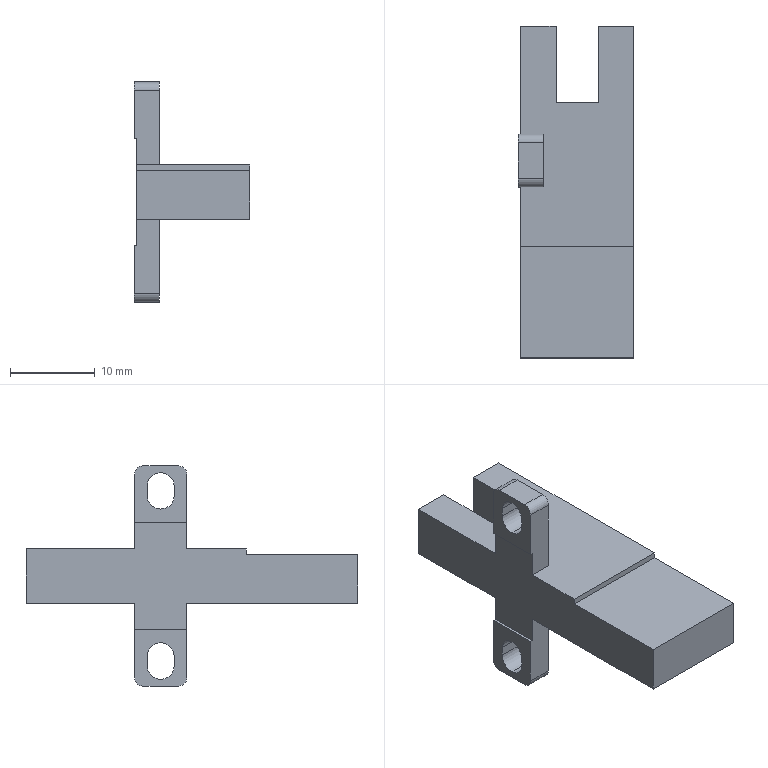Part | SolidWorks | features BaseBody 1 | 1 solid | 38 faces | box 13.7 x 39.2 x 26 mm | volume 3231 mm3 | plane 28 | cylinder 10 | commonest cylinder face diameters 3.2 x6 2 x4
STEP:
#1=CARTESIAN_POINT('',(-7.,6.3,-12.2));
#2=VERTEX_POINT('',#1);
#3=CARTESIAN_POINT('',(-7.,7.9,-10.6));
#4=VERTEX_POINT('',#3);
#5=CARTESIAN_POINT('',(-7.,6.3,-10.6));
#6=DIRECTION('',(1.,0.,0.));
#7=DIRECTION('',(0.,0.,-1.));
#8=AXIS2_PLACEMENT_3D('',#5,#6,#7);
#9=CIRCLE('',#8,1.6);
#10=EDGE_CURVE('',#2,#4,#9,.T.);
#11=ORIENTED_EDGE('',*,*,#10,.F.);
#12=CARTESIAN_POINT('',(-4.,6.3,-12.2));
#13=VERTEX_POINT('',#12);
#14=CARTESIAN_POINT('',(-4.,6.3,-12.2));
#15=DIRECTION('',(1.,0.,0.));
#16=VECTOR('',#15,1000.);
#17=LINE('',#14,#16);
#18=EDGE_CURVE('',#2,#13,#17,.T.);
#19=ORIENTED_EDGE('',*,*,#18,.T.);
#20=CARTESIAN_POINT('',(-4.,7.9,-10.6));
#21=VERTEX_POINT('',#20);
#22=CARTESIAN_POINT('',(-4.,6.3,-10.6));
#23=DIRECTION('',(-1.,0.,0.));
#24=DIRECTION('',(0.,0.,-1.));
#25=AXIS2_PLACEMENT_3D('',#22,#23,#24);
#26=CIRCLE('',#25,1.6);
#27=EDGE_CURVE('',#21,#13,#26,.T.);
#28=ORIENTED_EDGE('',*,*,#27,.F.);
#29=CARTESIAN_POINT('',(-4.,7.9,-10.6));
#30=DIRECTION('',(1.,0.,0.));
#31=VECTOR('',#30,1000.);
#32=LINE('',#29,#31);
#33=EDGE_CURVE('',#4,#21,#32,.T.);
#34=ORIENTED_EDGE('',*,*,#33,.F.);
#35=EDGE_LOOP('',(#11,#19,#28,#34));
#36=FACE_OUTER_BOUND('',#35,.T.);
#37=CARTESIAN_POINT('',(-4.,6.3,-10.6));
#38=DIRECTION('',(1.,0.,0.));
#39=DIRECTION('',(0.,0.,-1.));
#40=AXIS2_PLACEMENT_3D('',#37,#38,#39);
#41=CYLINDRICAL_SURFACE('',#40,1.6);
#42=ADVANCED_FACE('',(#36),#41,.F.);
#43=CARTESIAN_POINT('',(-7.,6.3,7.9));
#44=VERTEX_POINT('',#43);
#45=CARTESIAN_POINT('',(-7.,7.9,9.5));
#46=VERTEX_POINT('',#45);
#47=CARTESIAN_POINT('',(-7.,6.3,9.5));
#48=DIRECTION('',(1.,0.,0.));
#49=DIRECTION('',(0.,0.,-1.));
#50=AXIS2_PLACEMENT_3D('',#47,#48,#49);
#51=CIRCLE('',#50,1.6);
#52=EDGE_CURVE('',#44,#46,#51,.T.);
#53=ORIENTED_EDGE('',*,*,#52,.F.);
#54=CARTESIAN_POINT('',(-4.,6.3,7.9));
#55=VERTEX_POINT('',#54);
#56=CARTESIAN_POINT('',(-4.,6.3,7.9));
#57=DIRECTION('',(1.,0.,0.));
#58=VECTOR('',#57,1000.);
#59=LINE('',#56,#58);
#60=EDGE_CURVE('',#44,#55,#59,.T.);
#61=ORIENTED_EDGE('',*,*,#60,.T.);
#62=CARTESIAN_POINT('',(-4.,7.9,9.5));
#63=VERTEX_POINT('',#62);
#64=CARTESIAN_POINT('',(-4.,6.3,9.5));
#65=DIRECTION('',(-1.,0.,0.));
#66=DIRECTION('',(0.,0.,-1.));
#67=AXIS2_PLACEMENT_3D('',#64,#65,#66);
#68=CIRCLE('',#67,1.6);
#69=EDGE_CURVE('',#63,#55,#68,.T.);
#70=ORIENTED_EDGE('',*,*,#69,.F.);
#71=CARTESIAN_POINT('',(-4.,7.9,9.5));
#72=DIRECTION('',(1.,0.,0.));
#73=VECTOR('',#72,1000.);
#74=LINE('',#71,#73);
#75=EDGE_CURVE('',#46,#63,#74,.T.);
#76=ORIENTED_EDGE('',*,*,#75,.F.);
#77=EDGE_LOOP('',(#53,#61,#70,#76));
#78=FACE_OUTER_BOUND('',#77,.T.);
#79=CARTESIAN_POINT('',(-4.,6.3,9.5));
#80=DIRECTION('',(1.,0.,0.));
#81=DIRECTION('',(0.,0.,-1.));
#82=AXIS2_PLACEMENT_3D('',#79,#80,#81);
#83=CYLINDRICAL_SURFACE('',#82,1.6);
#84=ADVANCED_FACE('',(#78),#83,.F.);
#85=CARTESIAN_POINT('',(2.5,22.2,-3.2));
#86=VERTEX_POINT('',#85);
#87=CARTESIAN_POINT('',(2.5,13.2,-3.2));
#88=VERTEX_POINT('',#87);
#89=CARTESIAN_POINT('',(2.5,0.,-3.2));
#90=DIRECTION('',(0.,-1.,0.));
#91=VECTOR('',#90,1000.);
#92=LINE('',#89,#91);
#93=EDGE_CURVE('',#86,#88,#92,.T.);
#94=ORIENTED_EDGE('',*,*,#93,.F.);
#95=CARTESIAN_POINT('',(6.7,22.2,-3.2));
#96=VERTEX_POINT('',#95);
#97=CARTESIAN_POINT('',(0.,22.2,-3.2));
#98=DIRECTION('',(-1.,0.,0.));
#99=VECTOR('',#98,1000.);
#100=LINE('',#97,#99);
#101=EDGE_CURVE('',#96,#86,#100,.T.);
#102=ORIENTED_EDGE('',*,*,#101,.F.);
#103=CARTESIAN_POINT('',(6.7,-17.,-3.2));
#104=VERTEX_POINT('',#103);
#105=CARTESIAN_POINT('',(6.7,0.,-3.2));
#106=DIRECTION('',(0.,1.,0.));
#107=VECTOR('',#106,1000.);
#108=LINE('',#105,#107);
#109=EDGE_CURVE('',#104,#96,#108,.T.);
#110=ORIENTED_EDGE('',*,*,#109,.F.);
#111=CARTESIAN_POINT('',(-6.7,-17.,-3.2));
#112=VERTEX_POINT('',#111);
#113=CARTESIAN_POINT('',(0.,-17.,-3.2));
#114=DIRECTION('',(1.,0.,0.));
#115=VECTOR('',#114,1000.);
#116=LINE('',#113,#115);
#117=EDGE_CURVE('',#112,#104,#116,.T.);
#118=ORIENTED_EDGE('',*,*,#117,.F.);
#119=CARTESIAN_POINT('',(-6.7,3.2,-3.2));
#120=VERTEX_POINT('',#119);
#121=CARTESIAN_POINT('',(-6.7,0.,-3.2));
#122=DIRECTION('',(0.,-1.,0.));
#123=VECTOR('',#122,1000.);
#124=LINE('',#121,#123);
#125=EDGE_CURVE('',#120,#112,#124,.T.);
#126=ORIENTED_EDGE('',*,*,#125,.F.);
#127=CARTESIAN_POINT('',(-4.,3.2,-3.2));
#128=VERTEX_POINT('',#127);
#129=CARTESIAN_POINT('',(0.,3.2,-3.2));
#130=DIRECTION('',(-1.,0.,0.));
#131=VECTOR('',#130,1000.);
#132=LINE('',#129,#131);
#133=EDGE_CURVE('',#128,#120,#132,.T.);
#134=ORIENTED_EDGE('',*,*,#133,.F.);
#135=CARTESIAN_POINT('',(-4.,9.4,-3.2));
#136=VERTEX_POINT('',#135);
#137=CARTESIAN_POINT('',(-4.,0.,-3.2));
#138=DIRECTION('',(0.,-1.,0.));
#139=VECTOR('',#138,1000.);
#140=LINE('',#137,#139);
#141=EDGE_CURVE('',#136,#128,#140,.T.);
#142=ORIENTED_EDGE('',*,*,#141,.F.);
#143=CARTESIAN_POINT('',(-6.7,9.4,-3.2));
#144=VERTEX_POINT('',#143);
#145=CARTESIAN_POINT('',(0.,9.4,-3.2));
#146=DIRECTION('',(1.,0.,0.));
#147=VECTOR('',#146,1000.);
#148=LINE('',#145,#147);
#149=EDGE_CURVE('',#144,#136,#148,.T.);
#150=ORIENTED_EDGE('',*,*,#149,.F.);
#151=CARTESIAN_POINT('',(-6.7,22.2,-3.2));
#152=VERTEX_POINT('',#151);
#153=CARTESIAN_POINT('',(-6.7,0.,-3.2));
#154=DIRECTION('',(0.,-1.,0.));
#155=VECTOR('',#154,1000.);
#156=LINE('',#153,#155);
#157=EDGE_CURVE('',#152,#144,#156,.T.);
#158=ORIENTED_EDGE('',*,*,#157,.F.);
#159=CARTESIAN_POINT('',(-2.5,22.2,-3.2));
#160=VERTEX_POINT('',#159);
#161=CARTESIAN_POINT('',(0.,22.2,-3.2));
#162=DIRECTION('',(-1.,0.,0.));
#163=VECTOR('',#162,1000.);
#164=LINE('',#161,#163);
#165=EDGE_CURVE('',#160,#152,#164,.T.);
#166=ORIENTED_EDGE('',*,*,#165,.F.);
#167=CARTESIAN_POINT('',(-2.5,13.2,-3.2));
#168=VERTEX_POINT('',#167);
#169=CARTESIAN_POINT('',(-2.5,0.,-3.2));
#170=DIRECTION('',(0.,1.,0.));
#171=VECTOR('',#170,1000.);
#172=LINE('',#169,#171);
#173=EDGE_CURVE('',#168,#160,#172,.T.);
#174=ORIENTED_EDGE('',*,*,#173,.F.);
#175=CARTESIAN_POINT('',(0.,13.2,-3.2));
#176=DIRECTION('',(-1.,0.,0.));
#177=VECTOR('',#176,1000.);
#178=LINE('',#175,#177);
#179=EDGE_CURVE('',#88,#168,#178,.T.);
#180=ORIENTED_EDGE('',*,*,#179,.F.);
#181=EDGE_LOOP('',(#94,#102,#110,#118,#126,#134,#142,#150,#158,#166,#174,#180));
#182=FACE_OUTER_BOUND('',#181,.T.);
#183=CARTESIAN_POINT('',(0.,0.,-3.2));
#184=DIRECTION('',(0.,0.,1.));
#185=DIRECTION('',(1.,0.,0.));
#186=AXIS2_PLACEMENT_3D('',#183,#184,#185);
#187=PLANE('',#186);
#188=ADVANCED_FACE('',(#182),#187,.F.);
#189=CARTESIAN_POINT('',(2.5,13.2,3.2));
#190=VERTEX_POINT('',#189);
#191=CARTESIAN_POINT('',(-2.5,13.2,3.2));
#192=VERTEX_POINT('',#191);
#193=CARTESIAN_POINT('',(-2.5,13.2,3.2));
#194=DIRECTION('',(-1.,0.,0.));
#195=VECTOR('',#194,1000.);
#196=LINE('',#193,#195);
#197=EDGE_CURVE('',#190,#192,#196,.T.);
#198=ORIENTED_EDGE('',*,*,#197,.F.);
#199=CARTESIAN_POINT('',(2.5,13.2,-13.));
#200=DIRECTION('',(0.,0.,1.));
#201=VECTOR('',#200,1000.);
#202=LINE('',#199,#201);
#203=EDGE_CURVE('',#88,#190,#202,.T.);
#204=ORIENTED_EDGE('',*,*,#203,.F.);
#205=ORIENTED_EDGE('',*,*,#179,.T.);
#206=CARTESIAN_POINT('',(-2.5,13.2,-13.));
#207=DIRECTION('',(0.,0.,-1.));
#208=VECTOR('',#207,1000.);
#209=LINE('',#206,#208);
#210=EDGE_CURVE('',#192,#168,#209,.T.);
#211=ORIENTED_EDGE('',*,*,#210,.F.);
#212=EDGE_LOOP('',(#198,#204,#205,#211));
#213=FACE_OUTER_BOUND('',#212,.T.);
#214=CARTESIAN_POINT('',(-2.5,13.2,-13.));
#215=DIRECTION('',(0.,-1.,0.));
#216=DIRECTION('',(0.,0.,-1.));
#217=AXIS2_PLACEMENT_3D('',#214,#215,#216);
#218=PLANE('',#217);
#219=ADVANCED_FACE('',(#213),#218,.F.);
#220=CARTESIAN_POINT('',(2.5,22.2,3.2));
#221=VERTEX_POINT('',#220);
#222=CARTESIAN_POINT('',(2.5,13.2,3.2));
#223=DIRECTION('',(0.,-1.,0.));
#224=VECTOR('',#223,1000.);
#225=LINE('',#222,#224);
#226=EDGE_CURVE('',#221,#190,#225,.T.);
#227=ORIENTED_EDGE('',*,*,#226,.F.);
#228=CARTESIAN_POINT('',(2.5,22.2,-13.));
#229=DIRECTION('',(0.,0.,1.));
#230=VECTOR('',#229,1000.);
#231=LINE('',#228,#230);
#232=EDGE_CURVE('',#86,#221,#231,.T.);
#233=ORIENTED_EDGE('',*,*,#232,.F.);
#234=ORIENTED_EDGE('',*,*,#93,.T.);
#235=ORIENTED_EDGE('',*,*,#203,.T.);
#236=EDGE_LOOP('',(#227,#233,#234,#235));
#237=FACE_OUTER_BOUND('',#236,.T.);
#238=CARTESIAN_POINT('',(2.5,13.2,-13.));
#239=DIRECTION('',(1.,0.,0.));
#240=DIRECTION('',(0.,1.,0.));
#241=AXIS2_PLACEMENT_3D('',#238,#239,#240);
#242=PLANE('',#241);
#243=ADVANCED_FACE('',(#237),#242,.F.);
#244=CARTESIAN_POINT('',(6.7,22.2,3.2));
#245=VERTEX_POINT('',#244);
#246=CARTESIAN_POINT('',(6.7,22.2,-3.2));
#247=DIRECTION('',(0.,0.,-1.));
#248=VECTOR('',#247,1000.);
#249=LINE('',#246,#248);
#250=EDGE_CURVE('',#245,#96,#249,.T.);
#251=ORIENTED_EDGE('',*,*,#250,.T.);
#252=ORIENTED_EDGE('',*,*,#101,.T.);
#253=ORIENTED_EDGE('',*,*,#232,.T.);
#254=CARTESIAN_POINT('',(-2.5,22.2,3.2));
#255=DIRECTION('',(1.,0.,0.));
#256=VECTOR('',#255,1000.);
#257=LINE('',#254,#256);
#258=EDGE_CURVE('',#221,#245,#257,.T.);
#259=ORIENTED_EDGE('',*,*,#258,.T.);
#260=EDGE_LOOP('',(#251,#252,#253,#259));
#261=FACE_OUTER_BOUND('',#260,.T.);
#262=CARTESIAN_POINT('',(-2.5,22.2,-3.2));
#263=DIRECTION('',(0.,1.,0.));
#264=DIRECTION('',(0.,0.,1.));
#265=AXIS2_PLACEMENT_3D('',#262,#263,#264);
#266=PLANE('',#265);
#267=ADVANCED_FACE('',(#261),#266,.T.);
#268=ORIENTED_EDGE('',*,*,#250,.F.);
#269=CARTESIAN_POINT('',(6.7,-3.8,3.2));
#270=VERTEX_POINT('',#269);
#271=CARTESIAN_POINT('',(6.7,0.,3.2));
#272=DIRECTION('',(0.,-1.,0.));
#273=VECTOR('',#272,1000.);
#274=LINE('',#271,#273);
#275=EDGE_CURVE('',#245,#270,#274,.T.);
#276=ORIENTED_EDGE('',*,*,#275,.T.);
#277=CARTESIAN_POINT('',(6.7,-3.8,2.5));
#278=VERTEX_POINT('',#277);
#279=CARTESIAN_POINT('',(6.7,-3.8,3.2));
#280=DIRECTION('',(0.,0.,1.));
#281=VECTOR('',#280,1000.);
#282=LINE('',#279,#281);
#283=EDGE_CURVE('',#278,#270,#282,.T.);
#284=ORIENTED_EDGE('',*,*,#283,.F.);
#285=CARTESIAN_POINT('',(6.7,-17.,2.5));
#286=VERTEX_POINT('',#285);
#287=CARTESIAN_POINT('',(6.7,0.,2.5));
#288=DIRECTION('',(0.,-1.,0.));
#289=VECTOR('',#288,1000.);
#290=LINE('',#287,#289);
#291=EDGE_CURVE('',#278,#286,#290,.T.);
#292=ORIENTED_EDGE('',*,*,#291,.T.);
#293=CARTESIAN_POINT('',(6.7,-17.,-3.2));
#294=DIRECTION('',(0.,0.,-1.));
#295=VECTOR('',#294,1000.);
#296=LINE('',#293,#295);
#297=EDGE_CURVE('',#286,#104,#296,.T.);
#298=ORIENTED_EDGE('',*,*,#297,.T.);
#299=ORIENTED_EDGE('',*,*,#109,.T.);
#300=EDGE_LOOP('',(#268,#276,#284,#292,#298,#299));
#301=FACE_OUTER_BOUND('',#300,.T.);
#302=CARTESIAN_POINT('',(6.7,0.,-3.2));
#303=DIRECTION('',(1.,0.,0.));
#304=DIRECTION('',(0.,0.,-1.));
#305=AXIS2_PLACEMENT_3D('',#302,#303,#304);
#306=PLANE('',#305);
#307=ADVANCED_FACE('',(#301),#306,.T.);
#308=ORIENTED_EDGE('',*,*,#297,.F.);
#309=CARTESIAN_POINT('',(-6.7,-17.,2.5));
#310=VERTEX_POINT('',#309);
#311=CARTESIAN_POINT('',(0.,-17.,2.5));
#312=DIRECTION('',(-1.,0.,0.));
#313=VECTOR('',#312,1000.);
#314=LINE('',#311,#313);
#315=EDGE_CURVE('',#286,#310,#314,.T.);
#316=ORIENTED_EDGE('',*,*,#315,.T.);
#317=CARTESIAN_POINT('',(-6.7,-17.,0.));
#318=DIRECTION('',(0.,0.,-1.));
#319=VECTOR('',#318,1000.);
#320=LINE('',#317,#319);
#321=EDGE_CURVE('',#310,#112,#320,.T.);
#322=ORIENTED_EDGE('',*,*,#321,.T.);
#323=ORIENTED_EDGE('',*,*,#117,.T.);
#324=EDGE_LOOP('',(#308,#316,#322,#323));
#325=FACE_OUTER_BOUND('',#324,.T.);
#326=CARTESIAN_POINT('',(0.,-17.,0.));
#327=DIRECTION('',(0.,-1.,0.));
#328=DIRECTION('',(0.,0.,-1.));
#329=AXIS2_PLACEMENT_3D('',#326,#327,#328);
#330=PLANE('',#329);
#331=ADVANCED_FACE('',(#325),#330,.T.);
#332=ORIENTED_EDGE('',*,*,#125,.T.);
#333=ORIENTED_EDGE('',*,*,#321,.F.);
#334=CARTESIAN_POINT('',(-6.7,-3.8,2.5));
#335=VERTEX_POINT('',#334);
#336=CARTESIAN_POINT('',(-6.7,22.2,2.5));
#337=DIRECTION('',(0.,1.,0.));
#338=VECTOR('',#337,1000.);
#339=LINE('',#336,#338);
#340=EDGE_CURVE('',#310,#335,#339,.T.);
#341=ORIENTED_EDGE('',*,*,#340,.T.);
#342=CARTESIAN_POINT('',(-6.7,-3.8,3.2));
#343=VERTEX_POINT('',#342);
#344=CARTESIAN_POINT('',(-6.7,-3.8,3.2));
#345=DIRECTION('',(0.,0.,-1.));
#346=VECTOR('',#345,1000.);
#347=LINE('',#344,#346);
#348=EDGE_CURVE('',#343,#335,#347,.T.);
#349=ORIENTED_EDGE('',*,*,#348,.F.);
#350=CARTESIAN_POINT('',(-6.7,3.2,3.2));
#351=VERTEX_POINT('',#350);
#352=CARTESIAN_POINT('',(-6.7,22.2,3.2));
#353=DIRECTION('',(0.,1.,0.));
#354=VECTOR('',#353,1000.);
#355=LINE('',#352,#354);
#356=EDGE_CURVE('',#343,#351,#355,.T.);
#357=ORIENTED_EDGE('',*,*,#356,.T.);
#358=CARTESIAN_POINT('',(-6.7,3.2,6.3));
#359=VERTEX_POINT('',#358);
#360=CARTESIAN_POINT('',(-6.7,3.2,-3.2));
#361=DIRECTION('',(0.,0.,1.));
#362=VECTOR('',#361,1000.);
#363=LINE('',#360,#362);
#364=EDGE_CURVE('',#351,#359,#363,.T.);
#365=ORIENTED_EDGE('',*,*,#364,.T.);
#366=CARTESIAN_POINT('',(-6.7,9.4,6.3));
#367=VERTEX_POINT('',#366);
#368=CARTESIAN_POINT('',(-6.7,22.2,6.3));
#369=DIRECTION('',(0.,1.,0.));
#370=VECTOR('',#369,1000.);
#371=LINE('',#368,#370);
#372=EDGE_CURVE('',#359,#367,#371,.T.);
#373=ORIENTED_EDGE('',*,*,#372,.T.);
#374=CARTESIAN_POINT('',(-6.7,9.4,3.2));
#375=VERTEX_POINT('',#374);
#376=CARTESIAN_POINT('',(-6.7,9.4,-3.2));
#377=DIRECTION('',(0.,0.,-1.));
#378=VECTOR('',#377,1000.);
#379=LINE('',#376,#378);
#380=EDGE_CURVE('',#367,#375,#379,.T.);
#381=ORIENTED_EDGE('',*,*,#380,.T.);
#382=CARTESIAN_POINT('',(-6.7,22.2,3.2));
#383=VERTEX_POINT('',#382);
#384=CARTESIAN_POINT('',(-6.7,22.2,3.2));
#385=DIRECTION('',(0.,1.,0.));
#386=VECTOR('',#385,1000.);
#387=LINE('',#384,#386);
#388=EDGE_CURVE('',#375,#383,#387,.T.);
#389=ORIENTED_EDGE('',*,*,#388,.T.);
#390=CARTESIAN_POINT('',(-6.7,22.2,-3.2));
#391=DIRECTION('',(0.,0.,-1.));
#392=VECTOR('',#391,1000.);
#393=LINE('',#390,#392);
#394=EDGE_CURVE('',#383,#152,#393,.T.);
#395=ORIENTED_EDGE('',*,*,#394,.T.);
#396=ORIENTED_EDGE('',*,*,#157,.T.);
#397=CARTESIAN_POINT('',(-6.7,9.4,-6.3));
#398=VERTEX_POINT('',#397);
#399=CARTESIAN_POINT('',(-6.7,9.4,-3.2));
#400=DIRECTION('',(0.,0.,-1.));
#401=VECTOR('',#400,1000.);
#402=LINE('',#399,#401);
#403=EDGE_CURVE('',#144,#398,#402,.T.);
#404=ORIENTED_EDGE('',*,*,#403,.T.);
#405=CARTESIAN_POINT('',(-6.7,3.2,-6.3));
#406=VERTEX_POINT('',#405);
#407=CARTESIAN_POINT('',(-6.7,22.2,-6.3));
#408=DIRECTION('',(0.,-1.,0.));
#409=VECTOR('',#408,1000.);
#410=LINE('',#407,#409);
#411=EDGE_CURVE('',#398,#406,#410,.T.);
#412=ORIENTED_EDGE('',*,*,#411,.T.);
#413=CARTESIAN_POINT('',(-6.7,3.2,-3.2));
#414=DIRECTION('',(0.,0.,1.));
#415=VECTOR('',#414,1000.);
#416=LINE('',#413,#415);
#417=EDGE_CURVE('',#406,#120,#416,.T.);
#418=ORIENTED_EDGE('',*,*,#417,.T.);
#419=EDGE_LOOP('',(#332,#333,#341,#349,#357,#365,#373,#381,#389,#395,#396,#404,#412,#418));
#420=FACE_OUTER_BOUND('',#419,.T.);
#421=CARTESIAN_POINT('',(-6.7,22.2,-3.2));
#422=DIRECTION('',(-1.,0.,0.));
#423=DIRECTION('',(0.,0.,1.));
#424=AXIS2_PLACEMENT_3D('',#421,#422,#423);
#425=PLANE('',#424);
#426=ADVANCED_FACE('',(#420),#425,.T.);
#427=ORIENTED_EDGE('',*,*,#417,.F.);
#428=CARTESIAN_POINT('',(-7.,3.2,-6.3));
#429=VERTEX_POINT('',#428);
#430=CARTESIAN_POINT('',(0.,3.2,-6.3));
#431=DIRECTION('',(-1.,0.,0.));
#432=VECTOR('',#431,1000.);
#433=LINE('',#430,#432);
#434=EDGE_CURVE('',#406,#429,#433,.T.);
#435=ORIENTED_EDGE('',*,*,#434,.T.);
#436=CARTESIAN_POINT('',(-7.,3.2,-12.));
#437=VERTEX_POINT('',#436);
#438=CARTESIAN_POINT('',(-7.,3.2,-3.2));
#439=DIRECTION('',(0.,0.,-1.));
#440=VECTOR('',#439,1000.);
#441=LINE('',#438,#440);
#442=EDGE_CURVE('',#429,#437,#441,.T.);
#443=ORIENTED_EDGE('',*,*,#442,.T.);
#444=CARTESIAN_POINT('',(-4.,3.2,-12.));
#445=VERTEX_POINT('',#444);
#446=CARTESIAN_POINT('',(0.,3.2,-12.));
#447=DIRECTION('',(1.,0.,0.));
#448=VECTOR('',#447,1000.);
#449=LINE('',#446,#448);
#450=EDGE_CURVE('',#437,#445,#449,.T.);
#451=ORIENTED_EDGE('',*,*,#450,.T.);
#452=CARTESIAN_POINT('',(-4.,3.2,-3.2));
#453=DIRECTION('',(0.,0.,1.));
#454=VECTOR('',#453,1000.);
#455=LINE('',#452,#454);
#456=EDGE_CURVE('',#445,#128,#455,.T.);
#457=ORIENTED_EDGE('',*,*,#456,.T.);
#458=ORIENTED_EDGE('',*,*,#133,.T.);
#459=EDGE_LOOP('',(#427,#435,#443,#451,#457,#458));
#460=FACE_OUTER_BOUND('',#459,.T.);
#461=CARTESIAN_POINT('',(0.,3.2,-3.2));
#462=DIRECTION('',(0.,-1.,0.));
#463=DIRECTION('',(0.,0.,-1.));
#464=AXIS2_PLACEMENT_3D('',#461,#462,#463);
#465=PLANE('',#464);
#466=ADVANCED_FACE('',(#460),#465,.T.);
#467=ORIENTED_EDGE('',*,*,#456,.F.);
#468=CARTESIAN_POINT('',(-4.,4.2,-13.));
#469=VERTEX_POINT('',#468);
#470=CARTESIAN_POINT('',(-4.,4.2,-12.));
#471=DIRECTION('',(1.,0.,0.));
#472=DIRECTION('',(0.,0.,-1.));
#473=AXIS2_PLACEMENT_3D('',#470,#471,#472);
#474=CIRCLE('',#473,1.);
#475=EDGE_CURVE('',#445,#469,#474,.T.);
#476=ORIENTED_EDGE('',*,*,#475,.T.);
#477=CARTESIAN_POINT('',(-4.,8.4,-13.));
#478=VERTEX_POINT('',#477);
#479=CARTESIAN_POINT('',(-4.,9.4,-13.));
#480=DIRECTION('',(0.,1.,0.));
#481=VECTOR('',#480,1000.);
#482=LINE('',#479,#481);
#483=EDGE_CURVE('',#469,#478,#482,.T.);
#484=ORIENTED_EDGE('',*,*,#483,.T.);
#485=CARTESIAN_POINT('',(-4.,9.4,-12.));
#486=VERTEX_POINT('',#485);
#487=CARTESIAN_POINT('',(-4.,8.4,-12.));
#488=DIRECTION('',(-1.,0.,0.));
#489=DIRECTION('',(0.,0.,1.));
#490=AXIS2_PLACEMENT_3D('',#487,#488,#489);
#491=CIRCLE('',#490,1.);
#492=EDGE_CURVE('',#486,#478,#491,.T.);
#493=ORIENTED_EDGE('',*,*,#492,.F.);
#494=CARTESIAN_POINT('',(-4.,9.4,-13.));
#495=DIRECTION('',(0.,0.,1.));
#496=VECTOR('',#495,1000.);
#497=LINE('',#494,#496);
#498=EDGE_CURVE('',#486,#136,#497,.T.);
#499=ORIENTED_EDGE('',*,*,#498,.T.);
#500=ORIENTED_EDGE('',*,*,#141,.T.);
#501=EDGE_LOOP('',(#467,#476,#484,#493,#499,#500));
#502=FACE_OUTER_BOUND('',#501,.T.);
#503=ORIENTED_EDGE('',*,*,#27,.T.);
#504=CARTESIAN_POINT('',(-4.,4.7,-10.6));
#505=VERTEX_POINT('',#504);
#506=CARTESIAN_POINT('',(-4.,6.3,-10.6));
#507=DIRECTION('',(-1.,0.,0.));
#508=DIRECTION('',(0.,0.,-1.));
#509=AXIS2_PLACEMENT_3D('',#506,#507,#508);
#510=CIRCLE('',#509,1.6);
#511=EDGE_CURVE('',#13,#505,#510,.T.);
#512=ORIENTED_EDGE('',*,*,#511,.T.);
#513=CARTESIAN_POINT('',(-4.,4.7,-9.5));
#514=VERTEX_POINT('',#513);
#515=CARTESIAN_POINT('',(-4.,4.7,-9.5));
#516=DIRECTION('',(0.,0.,1.));
#517=VECTOR('',#516,1000.);
#518=LINE('',#515,#517);
#519=EDGE_CURVE('',#505,#514,#518,.T.);
#520=ORIENTED_EDGE('',*,*,#519,.T.);
#521=CARTESIAN_POINT('',(-4.,7.9,-9.5));
#522=VERTEX_POINT('',#521);
#523=CARTESIAN_POINT('',(-4.,6.3,-9.5));
#524=DIRECTION('',(-1.,0.,0.));
#525=DIRECTION('',(0.,0.,-1.));
#526=AXIS2_PLACEMENT_3D('',#523,#524,#525);
#527=CIRCLE('',#526,1.6);
#528=EDGE_CURVE('',#514,#522,#527,.T.);
#529=ORIENTED_EDGE('',*,*,#528,.T.);
#530=CARTESIAN_POINT('',(-4.,7.9,-10.6));
#531=DIRECTION('',(0.,0.,-1.));
#532=VECTOR('',#531,1000.);
#533=LINE('',#530,#532);
#534=EDGE_CURVE('',#522,#21,#533,.T.);
#535=ORIENTED_EDGE('',*,*,#534,.T.);
#536=EDGE_LOOP('',(#503,#512,#520,#529,#535));
#537=FACE_BOUND('',#536,.T.);
#538=CARTESIAN_POINT('',(-4.,9.4,-13.));
#539=DIRECTION('',(1.,0.,0.));
#540=DIRECTION('',(0.,0.,-1.));
#541=AXIS2_PLACEMENT_3D('',#538,#539,#540);
#542=PLANE('',#541);
#543=ADVANCED_FACE('',(#502,#537),#542,.T.);
#544=ORIENTED_EDGE('',*,*,#403,.F.);
#545=ORIENTED_EDGE('',*,*,#149,.T.);
#546=ORIENTED_EDGE('',*,*,#498,.F.);
#547=CARTESIAN_POINT('',(-7.,9.4,-12.));
#548=VERTEX_POINT('',#547);
#549=CARTESIAN_POINT('',(0.,9.4,-12.));
#550=DIRECTION('',(1.,0.,0.));
#551=VECTOR('',#550,1000.);
#552=LINE('',#549,#551);
#553=EDGE_CURVE('',#548,#486,#552,.T.);
#554=ORIENTED_EDGE('',*,*,#553,.F.);
#555=CARTESIAN_POINT('',(-7.,9.4,-6.3));
#556=VERTEX_POINT('',#555);
#557=CARTESIAN_POINT('',(-7.,9.4,-3.2));
#558=DIRECTION('',(0.,0.,-1.));
#559=VECTOR('',#558,1000.);
#560=LINE('',#557,#559);
#561=EDGE_CURVE('',#556,#548,#560,.T.);
#562=ORIENTED_EDGE('',*,*,#561,.F.);
#563=CARTESIAN_POINT('',(0.,9.4,-6.3));
#564=DIRECTION('',(-1.,0.,0.));
#565=VECTOR('',#564,1000.);
#566=LINE('',#563,#565);
#567=EDGE_CURVE('',#398,#556,#566,.T.);
#568=ORIENTED_EDGE('',*,*,#567,.F.);
#569=EDGE_LOOP('',(#544,#545,#546,#554,#562,#568));
#570=FACE_OUTER_BOUND('',#569,.T.);
#571=CARTESIAN_POINT('',(0.,9.4,-3.2));
#572=DIRECTION('',(0.,-1.,0.));
#573=DIRECTION('',(0.,0.,-1.));
#574=AXIS2_PLACEMENT_3D('',#571,#572,#573);
#575=PLANE('',#574);
#576=ADVANCED_FACE('',(#570),#575,.F.);
#577=ORIENTED_EDGE('',*,*,#394,.F.);
#578=CARTESIAN_POINT('',(-2.5,22.2,3.2));
#579=VERTEX_POINT('',#578);
#580=CARTESIAN_POINT('',(-2.5,22.2,3.2));
#581=DIRECTION('',(1.,0.,0.));
#582=VECTOR('',#581,1000.);
#583=LINE('',#580,#582);
#584=EDGE_CURVE('',#383,#579,#583,.T.);
#585=ORIENTED_EDGE('',*,*,#584,.T.);
#586=CARTESIAN_POINT('',(-2.5,22.2,-3.2));
#587=DIRECTION('',(0.,0.,-1.));
#588=VECTOR('',#587,1000.);
#589=LINE('',#586,#588);
#590=EDGE_CURVE('',#579,#160,#589,.T.);
#591=ORIENTED_EDGE('',*,*,#590,.T.);
#592=ORIENTED_EDGE('',*,*,#165,.T.);
#593=EDGE_LOOP('',(#577,#585,#591,#592));
#594=FACE_OUTER_BOUND('',#593,.T.);
#595=CARTESIAN_POINT('',(-2.5,22.2,-3.2));
#596=DIRECTION('',(0.,1.,0.));
#597=DIRECTION('',(0.,0.,1.));
#598=AXIS2_PLACEMENT_3D('',#595,#596,#597);
#599=PLANE('',#598);
#600=ADVANCED_FACE('',(#594),#599,.T.);
#601=CARTESIAN_POINT('',(-2.5,22.2,3.2));
#602=DIRECTION('',(0.,1.,0.));
#603=VECTOR('',#602,1000.);
#604=LINE('',#601,#603);
#605=EDGE_CURVE('',#192,#579,#604,.T.);
#606=ORIENTED_EDGE('',*,*,#605,.F.);
#607=ORIENTED_EDGE('',*,*,#210,.T.);
#608=ORIENTED_EDGE('',*,*,#173,.T.);
#609=ORIENTED_EDGE('',*,*,#590,.F.);
#610=EDGE_LOOP('',(#606,#607,#608,#609));
#611=FACE_OUTER_BOUND('',#610,.T.);
#612=CARTESIAN_POINT('',(-2.5,22.2,-13.));
#613=DIRECTION('',(-1.,0.,0.));
#614=DIRECTION('',(0.,0.,1.));
#615=AXIS2_PLACEMENT_3D('',#612,#613,#614);
#616=PLANE('',#615);
#617=ADVANCED_FACE('',(#611),#616,.F.);
#618=ORIENTED_EDGE('',*,*,#275,.F.);
#619=ORIENTED_EDGE('',*,*,#258,.F.);
#620=ORIENTED_EDGE('',*,*,#226,.T.);
#621=ORIENTED_EDGE('',*,*,#197,.T.);
#622=ORIENTED_EDGE('',*,*,#605,.T.);
#623=ORIENTED_EDGE('',*,*,#584,.F.);
#624=ORIENTED_EDGE('',*,*,#388,.F.);
#625=CARTESIAN_POINT('',(-4.,9.4,3.2));
#626=VERTEX_POINT('',#625);
#627=CARTESIAN_POINT('',(0.,9.4,3.2));
#628=DIRECTION('',(1.,0.,0.));
#629=VECTOR('',#628,1000.);
#630=LINE('',#627,#629);
#631=EDGE_CURVE('',#375,#626,#630,.T.);
#632=ORIENTED_EDGE('',*,*,#631,.T.);
#633=CARTESIAN_POINT('',(-4.,3.2,3.2));
#634=VERTEX_POINT('',#633);
#635=CARTESIAN_POINT('',(-4.,0.,3.2));
#636=DIRECTION('',(0.,-1.,0.));
#637=VECTOR('',#636,1000.);
#638=LINE('',#635,#637);
#639=EDGE_CURVE('',#626,#634,#638,.T.);
#640=ORIENTED_EDGE('',*,*,#639,.T.);
#641=CARTESIAN_POINT('',(0.,3.2,3.2));
#642=DIRECTION('',(-1.,0.,0.));
#643=VECTOR('',#642,1000.);
#644=LINE('',#641,#643);
#645=EDGE_CURVE('',#634,#351,#644,.T.);
#646=ORIENTED_EDGE('',*,*,#645,.T.);
#647=ORIENTED_EDGE('',*,*,#356,.F.);
#648=CARTESIAN_POINT('',(0.,-3.8,3.2));
#649=DIRECTION('',(1.,0.,0.));
#650=VECTOR('',#649,1000.);
#651=LINE('',#648,#650);
#652=EDGE_CURVE('',#343,#270,#651,.T.);
#653=ORIENTED_EDGE('',*,*,#652,.T.);
#654=EDGE_LOOP('',(#618,#619,#620,#621,#622,#623,#624,#632,#640,#646,#647,#653));
#655=FACE_OUTER_BOUND('',#654,.T.);
#656=CARTESIAN_POINT('',(0.,0.,3.2));
#657=DIRECTION('',(0.,0.,1.));
#658=DIRECTION('',(1.,0.,0.));
#659=AXIS2_PLACEMENT_3D('',#656,#657,#658);
#660=PLANE('',#659);
#661=ADVANCED_FACE('',(#655),#660,.T.);
#662=ORIENTED_EDGE('',*,*,#340,.F.);
#663=ORIENTED_EDGE('',*,*,#315,.F.);
#664=ORIENTED_EDGE('',*,*,#291,.F.);
#665=CARTESIAN_POINT('',(-6.7,-3.8,2.5));
#666=DIRECTION('',(1.,0.,0.));
#667=VECTOR('',#666,1000.);
#668=LINE('',#665,#667);
#669=EDGE_CURVE('',#335,#278,#668,.T.);
#670=ORIENTED_EDGE('',*,*,#669,.F.);
#671=EDGE_LOOP('',(#662,#663,#664,#670));
#672=FACE_OUTER_BOUND('',#671,.T.);
#673=CARTESIAN_POINT('',(-6.7,-17.,2.5));
#674=DIRECTION('',(0.,0.,-1.));
#675=DIRECTION('',(-1.,0.,0.));
#676=AXIS2_PLACEMENT_3D('',#673,#674,#675);
#677=PLANE('',#676);
#678=ADVANCED_FACE('',(#672),#677,.F.);
#679=CARTESIAN_POINT('',(-7.,9.4,-6.3));
#680=DIRECTION('',(0.,-1.,0.));
#681=VECTOR('',#680,1000.);
#682=LINE('',#679,#681);
#683=EDGE_CURVE('',#556,#429,#682,.T.);
#684=ORIENTED_EDGE('',*,*,#683,.T.);
#685=ORIENTED_EDGE('',*,*,#434,.F.);
#686=ORIENTED_EDGE('',*,*,#411,.F.);
#687=ORIENTED_EDGE('',*,*,#567,.T.);
#688=EDGE_LOOP('',(#684,#685,#686,#687));
#689=FACE_OUTER_BOUND('',#688,.T.);
#690=CARTESIAN_POINT('',(-6.7,9.4,-6.3));
#691=DIRECTION('',(0.,0.,1.));
#692=DIRECTION('',(1.,0.,0.));
#693=AXIS2_PLACEMENT_3D('',#690,#691,#692);
#694=PLANE('',#693);
#695=ADVANCED_FACE('',(#689),#694,.T.);
#696=ORIENTED_EDGE('',*,*,#380,.F.);
#697=CARTESIAN_POINT('',(-7.,9.4,6.3));
#698=VERTEX_POINT('',#697);
#699=CARTESIAN_POINT('',(0.,9.4,6.3));
#700=DIRECTION('',(1.,0.,0.));
#701=VECTOR('',#700,1000.);
#702=LINE('',#699,#701);
#703=EDGE_CURVE('',#698,#367,#702,.T.);
#704=ORIENTED_EDGE('',*,*,#703,.F.);
#705=CARTESIAN_POINT('',(-7.,9.4,12.));
#706=VERTEX_POINT('',#705);
#707=CARTESIAN_POINT('',(-7.,9.4,-3.2));
#708=DIRECTION('',(0.,0.,-1.));
#709=VECTOR('',#708,1000.);
#710=LINE('',#707,#709);
#711=EDGE_CURVE('',#706,#698,#710,.T.);
#712=ORIENTED_EDGE('',*,*,#711,.F.);
#713=CARTESIAN_POINT('',(-4.,9.4,12.));
#714=VERTEX_POINT('',#713);
#715=CARTESIAN_POINT('',(0.,9.4,12.));
#716=DIRECTION('',(-1.,0.,0.));
#717=VECTOR('',#716,1000.);
#718=LINE('',#715,#717);
#719=EDGE_CURVE('',#714,#706,#718,.T.);
#720=ORIENTED_EDGE('',*,*,#719,.F.);
#721=CARTESIAN_POINT('',(-4.,9.4,-3.2));
#722=DIRECTION('',(0.,0.,1.));
#723=VECTOR('',#722,1000.);
#724=LINE('',#721,#723);
#725=EDGE_CURVE('',#626,#714,#724,.T.);
#726=ORIENTED_EDGE('',*,*,#725,.F.);
#727=ORIENTED_EDGE('',*,*,#631,.F.);
#728=EDGE_LOOP('',(#696,#704,#712,#720,#726,#727));
#729=FACE_OUTER_BOUND('',#728,.T.);
#730=CARTESIAN_POINT('',(0.,9.4,-3.2));
#731=DIRECTION('',(0.,-1.,0.));
#732=DIRECTION('',(0.,0.,-1.));
#733=AXIS2_PLACEMENT_3D('',#730,#731,#732);
#734=PLANE('',#733);
#735=ADVANCED_FACE('',(#729),#734,.F.);
#736=ORIENTED_EDGE('',*,*,#372,.F.);
#737=CARTESIAN_POINT('',(-7.,3.2,6.3));
#738=VERTEX_POINT('',#737);
#739=CARTESIAN_POINT('',(-7.,3.2,6.3));
#740=DIRECTION('',(-1.,0.,0.));
#741=VECTOR('',#740,1000.);
#742=LINE('',#739,#741);
#743=EDGE_CURVE('',#359,#738,#742,.T.);
#744=ORIENTED_EDGE('',*,*,#743,.T.);
#745=CARTESIAN_POINT('',(-7.,9.4,6.3));
#746=DIRECTION('',(0.,1.,0.));
#747=VECTOR('',#746,1000.);
#748=LINE('',#745,#747);
#749=EDGE_CURVE('',#738,#698,#748,.T.);
#750=ORIENTED_EDGE('',*,*,#749,.T.);
#751=ORIENTED_EDGE('',*,*,#703,.T.);
#752=EDGE_LOOP('',(#736,#744,#750,#751));
#753=FACE_OUTER_BOUND('',#752,.T.);
#754=CARTESIAN_POINT('',(-7.,9.4,6.3));
#755=DIRECTION('',(0.,0.,-1.));
#756=DIRECTION('',(-1.,0.,0.));
#757=AXIS2_PLACEMENT_3D('',#754,#755,#756);
#758=PLANE('',#757);
#759=ADVANCED_FACE('',(#753),#758,.T.);
#760=ORIENTED_EDGE('',*,*,#364,.F.);
#761=ORIENTED_EDGE('',*,*,#645,.F.);
#762=CARTESIAN_POINT('',(-4.,3.2,12.));
#763=VERTEX_POINT('',#762);
#764=CARTESIAN_POINT('',(-4.,3.2,-3.2));
#765=DIRECTION('',(0.,0.,1.));
#766=VECTOR('',#765,1000.);
#767=LINE('',#764,#766);
#768=EDGE_CURVE('',#634,#763,#767,.T.);
#769=ORIENTED_EDGE('',*,*,#768,.T.);
#770=CARTESIAN_POINT('',(-7.,3.2,12.));
#771=VERTEX_POINT('',#770);
#772=CARTESIAN_POINT('',(0.,3.2,12.));
#773=DIRECTION('',(-1.,0.,0.));
#774=VECTOR('',#773,1000.);
#775=LINE('',#772,#774);
#776=EDGE_CURVE('',#763,#771,#775,.T.);
#777=ORIENTED_EDGE('',*,*,#776,.T.);
#778=CARTESIAN_POINT('',(-7.,3.2,-3.2));
#779=DIRECTION('',(0.,0.,-1.));
#780=VECTOR('',#779,1000.);
#781=LINE('',#778,#780);
#782=EDGE_CURVE('',#771,#738,#781,.T.);
#783=ORIENTED_EDGE('',*,*,#782,.T.);
#784=ORIENTED_EDGE('',*,*,#743,.F.);
#785=EDGE_LOOP('',(#760,#761,#769,#777,#783,#784));
#786=FACE_OUTER_BOUND('',#785,.T.);
#787=CARTESIAN_POINT('',(0.,3.2,-3.2));
#788=DIRECTION('',(0.,-1.,0.));
#789=DIRECTION('',(0.,0.,-1.));
#790=AXIS2_PLACEMENT_3D('',#787,#788,#789);
#791=PLANE('',#790);
#792=ADVANCED_FACE('',(#786),#791,.T.);
#793=ORIENTED_EDGE('',*,*,#450,.F.);
#794=CARTESIAN_POINT('',(-7.,4.2,-13.));
#795=VERTEX_POINT('',#794);
#796=CARTESIAN_POINT('',(-7.,4.2,-12.));
#797=DIRECTION('',(1.,0.,0.));
#798=DIRECTION('',(0.,0.,-1.));
#799=AXIS2_PLACEMENT_3D('',#796,#797,#798);
#800=CIRCLE('',#799,1.);
#801=EDGE_CURVE('',#437,#795,#800,.T.);
#802=ORIENTED_EDGE('',*,*,#801,.T.);
#803=CARTESIAN_POINT('',(-24.859,4.2,-13.));
#804=DIRECTION('',(1.,0.,0.));
#805=VECTOR('',#804,1000.);
#806=LINE('',#803,#805);
#807=EDGE_CURVE('',#795,#469,#806,.T.);
#808=ORIENTED_EDGE('',*,*,#807,.T.);
#809=ORIENTED_EDGE('',*,*,#475,.F.);
#810=EDGE_LOOP('',(#793,#802,#808,#809));
#811=FACE_OUTER_BOUND('',#810,.T.);
#812=CARTESIAN_POINT('',(-24.859,4.2,-12.));
#813=DIRECTION('',(1.,0.,0.));
#814=DIRECTION('',(0.,0.,-1.));
#815=AXIS2_PLACEMENT_3D('',#812,#813,#814);
#816=CYLINDRICAL_SURFACE('',#815,1.);
#817=ADVANCED_FACE('',(#811),#816,.T.);
#818=ORIENTED_EDGE('',*,*,#442,.F.);
#819=ORIENTED_EDGE('',*,*,#683,.F.);
#820=ORIENTED_EDGE('',*,*,#561,.T.);
#821=CARTESIAN_POINT('',(-7.,8.4,-13.));
#822=VERTEX_POINT('',#821);
#823=CARTESIAN_POINT('',(-7.,8.4,-12.));
#824=DIRECTION('',(-1.,0.,0.));
#825=DIRECTION('',(0.,0.,1.));
#826=AXIS2_PLACEMENT_3D('',#823,#824,#825);
#827=CIRCLE('',#826,1.);
#828=EDGE_CURVE('',#548,#822,#827,.T.);
#829=ORIENTED_EDGE('',*,*,#828,.T.);
#830=CARTESIAN_POINT('',(-7.,9.4,-13.));
#831=DIRECTION('',(0.,-1.,0.));
#832=VECTOR('',#831,1000.);
#833=LINE('',#830,#832);
#834=EDGE_CURVE('',#822,#795,#833,.T.);
#835=ORIENTED_EDGE('',*,*,#834,.T.);
#836=ORIENTED_EDGE('',*,*,#801,.F.);
#837=EDGE_LOOP('',(#818,#819,#820,#829,#835,#836));
#838=FACE_OUTER_BOUND('',#837,.T.);
#839=CARTESIAN_POINT('',(-7.,7.9,-9.5));
#840=VERTEX_POINT('',#839);
#841=CARTESIAN_POINT('',(-7.,4.7,-9.5));
#842=VERTEX_POINT('',#841);
#843=CARTESIAN_POINT('',(-7.,6.3,-9.5));
#844=DIRECTION('',(1.,0.,0.));
#845=DIRECTION('',(0.,0.,-1.));
#846=AXIS2_PLACEMENT_3D('',#843,#844,#845);
#847=CIRCLE('',#846,1.6);
#848=EDGE_CURVE('',#840,#842,#847,.T.);
#849=ORIENTED_EDGE('',*,*,#848,.T.);
#850=CARTESIAN_POINT('',(-7.,4.7,-10.6));
#851=VERTEX_POINT('',#850);
#852=CARTESIAN_POINT('',(-7.,4.7,-9.5));
#853=DIRECTION('',(0.,0.,-1.));
#854=VECTOR('',#853,1000.);
#855=LINE('',#852,#854);
#856=EDGE_CURVE('',#842,#851,#855,.T.);
#857=ORIENTED_EDGE('',*,*,#856,.T.);
#858=CARTESIAN_POINT('',(-7.,6.3,-10.6));
#859=DIRECTION('',(1.,0.,0.));
#860=DIRECTION('',(0.,0.,-1.));
#861=AXIS2_PLACEMENT_3D('',#858,#859,#860);
#862=CIRCLE('',#861,1.6);
#863=EDGE_CURVE('',#851,#2,#862,.T.);
#864=ORIENTED_EDGE('',*,*,#863,.T.);
#865=ORIENTED_EDGE('',*,*,#10,.T.);
#866=CARTESIAN_POINT('',(-7.,7.9,-10.6));
#867=DIRECTION('',(0.,0.,1.));
#868=VECTOR('',#867,1000.);
#869=LINE('',#866,#868);
#870=EDGE_CURVE('',#4,#840,#869,.T.);
#871=ORIENTED_EDGE('',*,*,#870,.T.);
#872=EDGE_LOOP('',(#849,#857,#864,#865,#871));
#873=FACE_BOUND('',#872,.T.);
#874=CARTESIAN_POINT('',(-7.,9.4,-6.3));
#875=DIRECTION('',(-1.,0.,0.));
#876=DIRECTION('',(0.,0.,1.));
#877=AXIS2_PLACEMENT_3D('',#874,#875,#876);
#878=PLANE('',#877);
#879=ADVANCED_FACE('',(#838,#873),#878,.T.);
#880=ORIENTED_EDGE('',*,*,#483,.F.);
#881=ORIENTED_EDGE('',*,*,#807,.F.);
#882=ORIENTED_EDGE('',*,*,#834,.F.);
#883=CARTESIAN_POINT('',(-7.,8.4,-13.));
#884=DIRECTION('',(1.,0.,0.));
#885=VECTOR('',#884,1000.);
#886=LINE('',#883,#885);
#887=EDGE_CURVE('',#822,#478,#886,.T.);
#888=ORIENTED_EDGE('',*,*,#887,.T.);
#889=EDGE_LOOP('',(#880,#881,#882,#888));
#890=FACE_OUTER_BOUND('',#889,.T.);
#891=CARTESIAN_POINT('',(-7.,9.4,-13.));
#892=DIRECTION('',(0.,0.,-1.));
#893=DIRECTION('',(-1.,0.,0.));
#894=AXIS2_PLACEMENT_3D('',#891,#892,#893);
#895=PLANE('',#894);
#896=ADVANCED_FACE('',(#890),#895,.T.);
#897=ORIENTED_EDGE('',*,*,#18,.F.);
#898=ORIENTED_EDGE('',*,*,#863,.F.);
#899=CARTESIAN_POINT('',(-4.,4.7,-10.6));
#900=DIRECTION('',(-1.,0.,0.));
#901=VECTOR('',#900,1000.);
#902=LINE('',#899,#901);
#903=EDGE_CURVE('',#505,#851,#902,.T.);
#904=ORIENTED_EDGE('',*,*,#903,.F.);
#905=ORIENTED_EDGE('',*,*,#511,.F.);
#906=EDGE_LOOP('',(#897,#898,#904,#905));
#907=FACE_OUTER_BOUND('',#906,.T.);
#908=CARTESIAN_POINT('',(-4.,6.3,-10.6));
#909=DIRECTION('',(1.,0.,0.));
#910=DIRECTION('',(0.,0.,-1.));
#911=AXIS2_PLACEMENT_3D('',#908,#909,#910);
#912=CYLINDRICAL_SURFACE('',#911,1.6);
#913=ADVANCED_FACE('',(#907),#912,.F.);
#914=CARTESIAN_POINT('',(-4.,7.9,-9.5));
#915=DIRECTION('',(-1.,0.,0.));
#916=VECTOR('',#915,1000.);
#917=LINE('',#914,#916);
#918=EDGE_CURVE('',#522,#840,#917,.T.);
#919=ORIENTED_EDGE('',*,*,#918,.F.);
#920=ORIENTED_EDGE('',*,*,#528,.F.);
#921=CARTESIAN_POINT('',(-4.,4.7,-9.5));
#922=DIRECTION('',(1.,0.,0.));
#923=VECTOR('',#922,1000.);
#924=LINE('',#921,#923);
#925=EDGE_CURVE('',#842,#514,#924,.T.);
#926=ORIENTED_EDGE('',*,*,#925,.F.);
#927=ORIENTED_EDGE('',*,*,#848,.F.);
#928=EDGE_LOOP('',(#919,#920,#926,#927));
#929=FACE_OUTER_BOUND('',#928,.T.);
#930=CARTESIAN_POINT('',(-4.,6.3,-9.5));
#931=DIRECTION('',(1.,0.,0.));
#932=DIRECTION('',(0.,0.,-1.));
#933=AXIS2_PLACEMENT_3D('',#930,#931,#932);
#934=CYLINDRICAL_SURFACE('',#933,1.6);
#935=ADVANCED_FACE('',(#929),#934,.F.);
#936=ORIENTED_EDGE('',*,*,#553,.T.);
#937=ORIENTED_EDGE('',*,*,#492,.T.);
#938=ORIENTED_EDGE('',*,*,#887,.F.);
#939=ORIENTED_EDGE('',*,*,#828,.F.);
#940=EDGE_LOOP('',(#936,#937,#938,#939));
#941=FACE_OUTER_BOUND('',#940,.T.);
#942=CARTESIAN_POINT('',(24.559,8.4,-12.));
#943=DIRECTION('',(-1.,0.,0.));
#944=DIRECTION('',(0.,0.,1.));
#945=AXIS2_PLACEMENT_3D('',#942,#943,#944);
#946=CYLINDRICAL_SURFACE('',#945,1.);
#947=ADVANCED_FACE('',(#941),#946,.T.);
#948=ORIENTED_EDGE('',*,*,#669,.T.);
#949=ORIENTED_EDGE('',*,*,#283,.T.);
#950=ORIENTED_EDGE('',*,*,#652,.F.);
#951=ORIENTED_EDGE('',*,*,#348,.T.);
#952=EDGE_LOOP('',(#948,#949,#950,#951));
#953=FACE_OUTER_BOUND('',#952,.T.);
#954=CARTESIAN_POINT('',(-6.7,-3.8,3.2));
#955=DIRECTION('',(0.,-1.,0.));
#956=DIRECTION('',(0.,0.,-1.));
#957=AXIS2_PLACEMENT_3D('',#954,#955,#956);
#958=PLANE('',#957);
#959=ADVANCED_FACE('',(#953),#958,.T.);
#960=ORIENTED_EDGE('',*,*,#725,.T.);
#961=CARTESIAN_POINT('',(-4.,8.4,13.));
#962=VERTEX_POINT('',#961);
#963=CARTESIAN_POINT('',(-4.,8.4,12.));
#964=DIRECTION('',(1.,0.,0.));
#965=DIRECTION('',(0.,0.,-1.));
#966=AXIS2_PLACEMENT_3D('',#963,#964,#965);
#967=CIRCLE('',#966,1.);
#968=EDGE_CURVE('',#714,#962,#967,.T.);
#969=ORIENTED_EDGE('',*,*,#968,.T.);
#970=CARTESIAN_POINT('',(-4.,4.2,13.));
#971=VERTEX_POINT('',#970);
#972=CARTESIAN_POINT('',(-4.,9.4,13.));
#973=DIRECTION('',(0.,-1.,0.));
#974=VECTOR('',#973,1000.);
#975=LINE('',#972,#974);
#976=EDGE_CURVE('',#962,#971,#975,.T.);
#977=ORIENTED_EDGE('',*,*,#976,.T.);
#978=CARTESIAN_POINT('',(-4.,4.2,12.));
#979=DIRECTION('',(1.,0.,0.));
#980=DIRECTION('',(0.,0.,1.));
#981=AXIS2_PLACEMENT_3D('',#978,#979,#980);
#982=CIRCLE('',#981,1.);
#983=EDGE_CURVE('',#971,#763,#982,.T.);
#984=ORIENTED_EDGE('',*,*,#983,.T.);
#985=ORIENTED_EDGE('',*,*,#768,.F.);
#986=ORIENTED_EDGE('',*,*,#639,.F.);
#987=EDGE_LOOP('',(#960,#969,#977,#984,#985,#986));
#988=FACE_OUTER_BOUND('',#987,.T.);
#989=CARTESIAN_POINT('',(-4.,7.9,10.6));
#990=VERTEX_POINT('',#989);
#991=CARTESIAN_POINT('',(-4.,7.9,9.5));
#992=DIRECTION('',(0.,0.,-1.));
#993=VECTOR('',#992,1000.);
#994=LINE('',#991,#993);
#995=EDGE_CURVE('',#990,#63,#994,.T.);
#996=ORIENTED_EDGE('',*,*,#995,.T.);
#997=ORIENTED_EDGE('',*,*,#69,.T.);
#998=CARTESIAN_POINT('',(-4.,4.7,9.5));
#999=VERTEX_POINT('',#998);
#1000=CARTESIAN_POINT('',(-4.,6.3,9.5));
#1001=DIRECTION('',(-1.,0.,0.));
#1002=DIRECTION('',(0.,0.,-1.));
#1003=AXIS2_PLACEMENT_3D('',#1000,#1001,#1002);
#1004=CIRCLE('',#1003,1.6);
#1005=EDGE_CURVE('',#55,#999,#1004,.T.);
#1006=ORIENTED_EDGE('',*,*,#1005,.T.);
#1007=CARTESIAN_POINT('',(-4.,4.7,10.6));
#1008=VERTEX_POINT('',#1007);
#1009=CARTESIAN_POINT('',(-4.,4.7,10.6));
#1010=DIRECTION('',(0.,0.,1.));
#1011=VECTOR('',#1010,1000.);
#1012=LINE('',#1009,#1011);
#1013=EDGE_CURVE('',#999,#1008,#1012,.T.);
#1014=ORIENTED_EDGE('',*,*,#1013,.T.);
#1015=CARTESIAN_POINT('',(-4.,6.3,10.6));
#1016=DIRECTION('',(-1.,0.,0.));
#1017=DIRECTION('',(0.,0.,-1.));
#1018=AXIS2_PLACEMENT_3D('',#1015,#1016,#1017);
#1019=CIRCLE('',#1018,1.6);
#1020=EDGE_CURVE('',#1008,#990,#1019,.T.);
#1021=ORIENTED_EDGE('',*,*,#1020,.T.);
#1022=EDGE_LOOP('',(#996,#997,#1006,#1014,#1021));
#1023=FACE_BOUND('',#1022,.T.);
#1024=CARTESIAN_POINT('',(-4.,9.4,-13.));
#1025=DIRECTION('',(1.,0.,0.));
#1026=DIRECTION('',(0.,0.,-1.));
#1027=AXIS2_PLACEMENT_3D('',#1024,#1025,#1026);
#1028=PLANE('',#1027);
#1029=ADVANCED_FACE('',(#988,#1023),#1028,.T.);
#1030=ORIENTED_EDGE('',*,*,#711,.T.);
#1031=ORIENTED_EDGE('',*,*,#749,.F.);
#1032=ORIENTED_EDGE('',*,*,#782,.F.);
#1033=CARTESIAN_POINT('',(-7.,4.2,13.));
#1034=VERTEX_POINT('',#1033);
#1035=CARTESIAN_POINT('',(-7.,4.2,12.));
#1036=DIRECTION('',(-1.,0.,0.));
#1037=DIRECTION('',(0.,0.,1.));
#1038=AXIS2_PLACEMENT_3D('',#1035,#1036,#1037);
#1039=CIRCLE('',#1038,1.);
#1040=EDGE_CURVE('',#771,#1034,#1039,.T.);
#1041=ORIENTED_EDGE('',*,*,#1040,.T.);
#1042=CARTESIAN_POINT('',(-7.,8.4,13.));
#1043=VERTEX_POINT('',#1042);
#1044=CARTESIAN_POINT('',(-7.,9.4,13.));
#1045=DIRECTION('',(0.,1.,0.));
#1046=VECTOR('',#1045,1000.);
#1047=LINE('',#1044,#1046);
#1048=EDGE_CURVE('',#1034,#1043,#1047,.T.);
#1049=ORIENTED_EDGE('',*,*,#1048,.T.);
#1050=CARTESIAN_POINT('',(-7.,8.4,12.));
#1051=DIRECTION('',(-1.,0.,0.));
#1052=DIRECTION('',(0.,0.,-1.));
#1053=AXIS2_PLACEMENT_3D('',#1050,#1051,#1052);
#1054=CIRCLE('',#1053,1.);
#1055=EDGE_CURVE('',#1043,#706,#1054,.T.);
#1056=ORIENTED_EDGE('',*,*,#1055,.T.);
#1057=EDGE_LOOP('',(#1030,#1031,#1032,#1041,#1049,#1056));
#1058=FACE_OUTER_BOUND('',#1057,.T.);
#1059=CARTESIAN_POINT('',(-7.,4.7,10.6));
#1060=VERTEX_POINT('',#1059);
#1061=CARTESIAN_POINT('',(-7.,4.7,9.5));
#1062=VERTEX_POINT('',#1061);
#1063=CARTESIAN_POINT('',(-7.,4.7,10.6));
#1064=DIRECTION('',(0.,0.,-1.));
#1065=VECTOR('',#1064,1000.);
#1066=LINE('',#1063,#1065);
#1067=EDGE_CURVE('',#1060,#1062,#1066,.T.);
#1068=ORIENTED_EDGE('',*,*,#1067,.T.);
#1069=CARTESIAN_POINT('',(-7.,6.3,9.5));
#1070=DIRECTION('',(1.,0.,0.));
#1071=DIRECTION('',(0.,0.,-1.));
#1072=AXIS2_PLACEMENT_3D('',#1069,#1070,#1071);
#1073=CIRCLE('',#1072,1.6);
#1074=EDGE_CURVE('',#1062,#44,#1073,.T.);
#1075=ORIENTED_EDGE('',*,*,#1074,.T.);
#1076=ORIENTED_EDGE('',*,*,#52,.T.);
#1077=CARTESIAN_POINT('',(-7.,7.9,10.6));
#1078=VERTEX_POINT('',#1077);
#1079=CARTESIAN_POINT('',(-7.,7.9,9.5));
#1080=DIRECTION('',(0.,0.,1.));
#1081=VECTOR('',#1080,1000.);
#1082=LINE('',#1079,#1081);
#1083=EDGE_CURVE('',#46,#1078,#1082,.T.);
#1084=ORIENTED_EDGE('',*,*,#1083,.T.);
#1085=CARTESIAN_POINT('',(-7.,6.3,10.6));
#1086=DIRECTION('',(1.,0.,0.));
#1087=DIRECTION('',(0.,0.,-1.));
#1088=AXIS2_PLACEMENT_3D('',#1085,#1086,#1087);
#1089=CIRCLE('',#1088,1.6);
#1090=EDGE_CURVE('',#1078,#1060,#1089,.T.);
#1091=ORIENTED_EDGE('',*,*,#1090,.T.);
#1092=EDGE_LOOP('',(#1068,#1075,#1076,#1084,#1091));
#1093=FACE_BOUND('',#1092,.T.);
#1094=CARTESIAN_POINT('',(-7.,9.4,13.));
#1095=DIRECTION('',(-1.,0.,0.));
#1096=DIRECTION('',(0.,0.,1.));
#1097=AXIS2_PLACEMENT_3D('',#1094,#1095,#1096);
#1098=PLANE('',#1097);
#1099=ADVANCED_FACE('',(#1058,#1093),#1098,.T.);
#1100=ORIENTED_EDGE('',*,*,#719,.T.);
#1101=ORIENTED_EDGE('',*,*,#1055,.F.);
#1102=CARTESIAN_POINT('',(-24.859,8.4,13.));
#1103=DIRECTION('',(1.,0.,0.));
#1104=VECTOR('',#1103,1000.);
#1105=LINE('',#1102,#1104);
#1106=EDGE_CURVE('',#1043,#962,#1105,.T.);
#1107=ORIENTED_EDGE('',*,*,#1106,.T.);
#1108=ORIENTED_EDGE('',*,*,#968,.F.);
#1109=EDGE_LOOP('',(#1100,#1101,#1107,#1108));
#1110=FACE_OUTER_BOUND('',#1109,.T.);
#1111=CARTESIAN_POINT('',(-24.859,8.4,12.));
#1112=DIRECTION('',(1.,0.,0.));
#1113=DIRECTION('',(0.,0.,-1.));
#1114=AXIS2_PLACEMENT_3D('',#1111,#1112,#1113);
#1115=CYLINDRICAL_SURFACE('',#1114,1.);
#1116=ADVANCED_FACE('',(#1110),#1115,.T.);
#1117=ORIENTED_EDGE('',*,*,#776,.F.);
#1118=ORIENTED_EDGE('',*,*,#983,.F.);
#1119=CARTESIAN_POINT('',(24.559,4.2,13.));
#1120=DIRECTION('',(-1.,0.,0.));
#1121=VECTOR('',#1120,1000.);
#1122=LINE('',#1119,#1121);
#1123=EDGE_CURVE('',#971,#1034,#1122,.T.);
#1124=ORIENTED_EDGE('',*,*,#1123,.T.);
#1125=ORIENTED_EDGE('',*,*,#1040,.F.);
#1126=EDGE_LOOP('',(#1117,#1118,#1124,#1125));
#1127=FACE_OUTER_BOUND('',#1126,.T.);
#1128=CARTESIAN_POINT('',(24.559,4.2,12.));
#1129=DIRECTION('',(-1.,0.,0.));
#1130=DIRECTION('',(0.,0.,1.));
#1131=AXIS2_PLACEMENT_3D('',#1128,#1129,#1130);
#1132=CYLINDRICAL_SURFACE('',#1131,1.);
#1133=ADVANCED_FACE('',(#1127),#1132,.T.);
#1134=ORIENTED_EDGE('',*,*,#925,.T.);
#1135=ORIENTED_EDGE('',*,*,#519,.F.);
#1136=ORIENTED_EDGE('',*,*,#903,.T.);
#1137=ORIENTED_EDGE('',*,*,#856,.F.);
#1138=EDGE_LOOP('',(#1134,#1135,#1136,#1137));
#1139=FACE_OUTER_BOUND('',#1138,.T.);
#1140=CARTESIAN_POINT('',(-4.,4.7,-9.5));
#1141=DIRECTION('',(0.,-1.,0.));
#1142=DIRECTION('',(0.,0.,-1.));
#1143=AXIS2_PLACEMENT_3D('',#1140,#1141,#1142);
#1144=PLANE('',#1143);
#1145=ADVANCED_FACE('',(#1139),#1144,.F.);
#1146=ORIENTED_EDGE('',*,*,#33,.T.);
#1147=ORIENTED_EDGE('',*,*,#534,.F.);
#1148=ORIENTED_EDGE('',*,*,#918,.T.);
#1149=ORIENTED_EDGE('',*,*,#870,.F.);
#1150=EDGE_LOOP('',(#1146,#1147,#1148,#1149));
#1151=FACE_OUTER_BOUND('',#1150,.T.);
#1152=CARTESIAN_POINT('',(-4.,7.9,-10.6));
#1153=DIRECTION('',(0.,1.,0.));
#1154=DIRECTION('',(0.,0.,1.));
#1155=AXIS2_PLACEMENT_3D('',#1152,#1153,#1154);
#1156=PLANE('',#1155);
#1157=ADVANCED_FACE('',(#1151),#1156,.F.);
#1158=ORIENTED_EDGE('',*,*,#976,.F.);
#1159=ORIENTED_EDGE('',*,*,#1106,.F.);
#1160=ORIENTED_EDGE('',*,*,#1048,.F.);
#1161=ORIENTED_EDGE('',*,*,#1123,.F.);
#1162=EDGE_LOOP('',(#1158,#1159,#1160,#1161));
#1163=FACE_OUTER_BOUND('',#1162,.T.);
#1164=CARTESIAN_POINT('',(-4.,9.4,13.));
#1165=DIRECTION('',(0.,0.,1.));
#1166=DIRECTION('',(1.,0.,0.));
#1167=AXIS2_PLACEMENT_3D('',#1164,#1165,#1166);
#1168=PLANE('',#1167);
#1169=ADVANCED_FACE('',(#1163),#1168,.T.);
#1170=ORIENTED_EDGE('',*,*,#60,.F.);
#1171=ORIENTED_EDGE('',*,*,#1074,.F.);
#1172=CARTESIAN_POINT('',(-4.,4.7,9.5));
#1173=DIRECTION('',(-1.,0.,0.));
#1174=VECTOR('',#1173,1000.);
#1175=LINE('',#1172,#1174);
#1176=EDGE_CURVE('',#999,#1062,#1175,.T.);
#1177=ORIENTED_EDGE('',*,*,#1176,.F.);
#1178=ORIENTED_EDGE('',*,*,#1005,.F.);
#1179=EDGE_LOOP('',(#1170,#1171,#1177,#1178));
#1180=FACE_OUTER_BOUND('',#1179,.T.);
#1181=CARTESIAN_POINT('',(-4.,6.3,9.5));
#1182=DIRECTION('',(1.,0.,0.));
#1183=DIRECTION('',(0.,0.,-1.));
#1184=AXIS2_PLACEMENT_3D('',#1181,#1182,#1183);
#1185=CYLINDRICAL_SURFACE('',#1184,1.6);
#1186=ADVANCED_FACE('',(#1180),#1185,.F.);
#1187=CARTESIAN_POINT('',(-4.,7.9,10.6));
#1188=DIRECTION('',(-1.,0.,0.));
#1189=VECTOR('',#1188,1000.);
#1190=LINE('',#1187,#1189);
#1191=EDGE_CURVE('',#990,#1078,#1190,.T.);
#1192=ORIENTED_EDGE('',*,*,#1191,.F.);
#1193=ORIENTED_EDGE('',*,*,#1020,.F.);
#1194=CARTESIAN_POINT('',(-4.,4.7,10.6));
#1195=DIRECTION('',(1.,0.,0.));
#1196=VECTOR('',#1195,1000.);
#1197=LINE('',#1194,#1196);
#1198=EDGE_CURVE('',#1060,#1008,#1197,.T.);
#1199=ORIENTED_EDGE('',*,*,#1198,.F.);
#1200=ORIENTED_EDGE('',*,*,#1090,.F.);
#1201=EDGE_LOOP('',(#1192,#1193,#1199,#1200));
#1202=FACE_OUTER_BOUND('',#1201,.T.);
#1203=CARTESIAN_POINT('',(-4.,6.3,10.6));
#1204=DIRECTION('',(1.,0.,0.));
#1205=DIRECTION('',(0.,0.,-1.));
#1206=AXIS2_PLACEMENT_3D('',#1203,#1204,#1205);
#1207=CYLINDRICAL_SURFACE('',#1206,1.6);
#1208=ADVANCED_FACE('',(#1202),#1207,.F.);
#1209=ORIENTED_EDGE('',*,*,#1198,.T.);
#1210=ORIENTED_EDGE('',*,*,#1013,.F.);
#1211=ORIENTED_EDGE('',*,*,#1176,.T.);
#1212=ORIENTED_EDGE('',*,*,#1067,.F.);
#1213=EDGE_LOOP('',(#1209,#1210,#1211,#1212));
#1214=FACE_OUTER_BOUND('',#1213,.T.);
#1215=CARTESIAN_POINT('',(-4.,4.7,10.6));
#1216=DIRECTION('',(0.,-1.,0.));
#1217=DIRECTION('',(0.,0.,-1.));
#1218=AXIS2_PLACEMENT_3D('',#1215,#1216,#1217);
#1219=PLANE('',#1218);
#1220=ADVANCED_FACE('',(#1214),#1219,.F.);
#1221=ORIENTED_EDGE('',*,*,#75,.T.);
#1222=ORIENTED_EDGE('',*,*,#995,.F.);
#1223=ORIENTED_EDGE('',*,*,#1191,.T.);
#1224=ORIENTED_EDGE('',*,*,#1083,.F.);
#1225=EDGE_LOOP('',(#1221,#1222,#1223,#1224));
#1226=FACE_OUTER_BOUND('',#1225,.T.);
#1227=CARTESIAN_POINT('',(-4.,7.9,9.5));
#1228=DIRECTION('',(0.,1.,0.));
#1229=DIRECTION('',(0.,0.,1.));
#1230=AXIS2_PLACEMENT_3D('',#1227,#1228,#1229);
#1231=PLANE('',#1230);
#1232=ADVANCED_FACE('',(#1226),#1231,.F.);
#1233=CLOSED_SHELL('',(#42,#84,#188,#219,#243,#267,#307,#331,#426,#466,#543,#576,#600,#617,#661,#678,#695,#735,#759,#792,#817,#879,#896,#913,#935,#947,#959,#1029,#1099,#1116,#1133,#1145,#1157,#1169,#1186,#1208,#1220,#1232));
#1234=MANIFOLD_SOLID_BREP('',#1233);
#1235=CARTESIAN_POINT('',(0.,0.,0.));
#1236=DIRECTION('',(0.,0.,1.));
#1237=DIRECTION('',(1.,0.,0.));
#1238=AXIS2_PLACEMENT_3D('',#1235,#1236,#1237);
#1239=(LENGTH_UNIT()NAMED_UNIT(*)SI_UNIT(.MILLI.,.METRE.));
#1240=UNCERTAINTY_MEASURE_WITH_UNIT(LENGTH_MEASURE(0.00001),#1239,'','');
#1241=(NAMED_UNIT(*)PLANE_ANGLE_UNIT()SI_UNIT($,.RADIAN.));
#1242=(NAMED_UNIT(*)SI_UNIT($,.STERADIAN.)SOLID_ANGLE_UNIT());
#1243=(GEOMETRIC_REPRESENTATION_CONTEXT(3)GLOBAL_UNCERTAINTY_ASSIGNED_CONTEXT((#1240))GLOBAL_UNIT_ASSIGNED_CONTEXT((#1239,#1241,#1242))REPRESENTATION_CONTEXT('',''));
#1244=ADVANCED_BREP_SHAPE_REPRESENTATION('',(#1234,#1238),#1243);